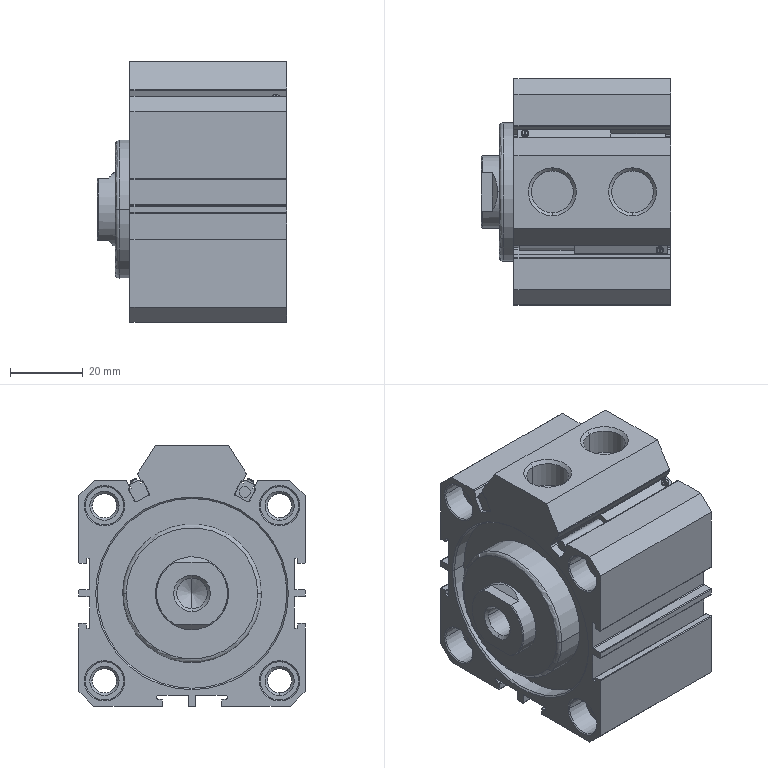Part | NX | features BREP 3 | 8 solids | 600 faces | box 52 x 62 x 71.5 mm | volume 290253 mm3 | cylinder 240 | plane 240 | cone 116 | torus 4 | commonest cylinder face diameters 0.4 x100 10.5 x32 0.8 x20 6.647 x16 0.6 x8 1 x8